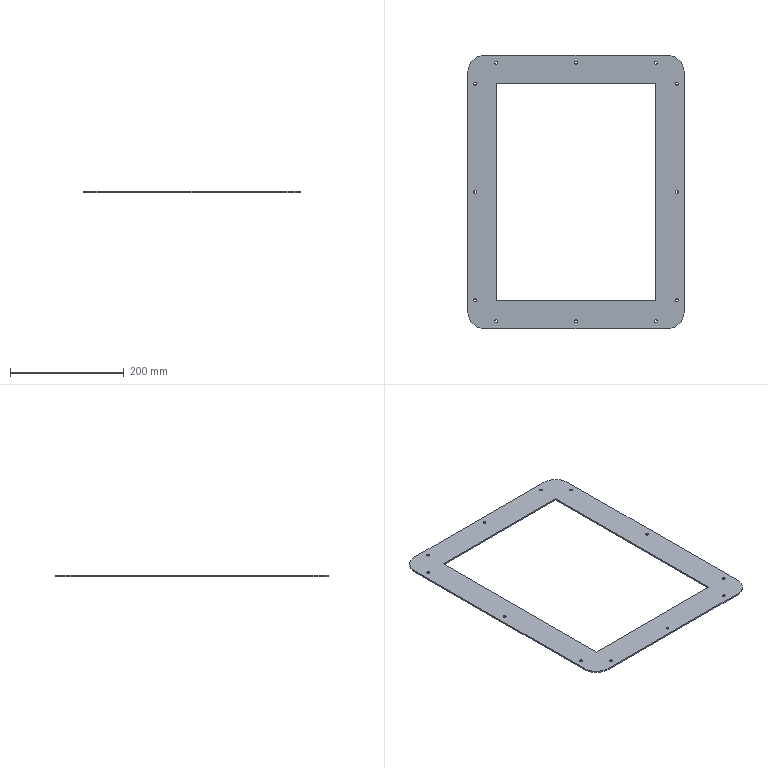Part | STEP file | HESS-408-70-15W-W-43-upper door closing plate 2 | 1 solid | 38 faces | box 380 x 480 x 2.5 mm | volume 187480 mm3 | cylinder 28 | plane 10 | commonest cylinder face diameters 5 x24 60 x4